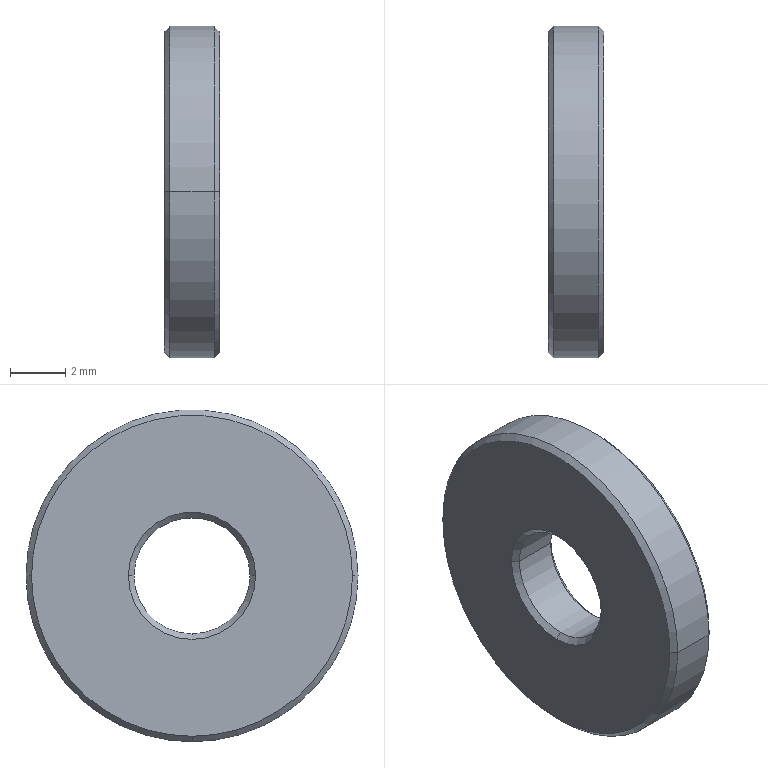Part | STEP file | BDQ-M4-D12-0.stp.STEP | 1 solid | 18 faces | box 2 x 12 x 12 mm | volume 196.45 mm3 | cone 12 | cylinder 4 | plane 2 | commonest cylinder face diameters 4.2 x2 12 x2
STEP:
#1=CARTESIAN_POINT('',(0.00000011,-2.3,0.));
#2=VERTEX_POINT('',#1);
#3=CARTESIAN_POINT('',(0.00000011,0.,-2.3));
#4=VERTEX_POINT('',#3);
#5=CARTESIAN_POINT('',(0.00000011,0.,0.));
#6=DIRECTION('',(1.,0.,0.));
#7=DIRECTION('',(0.,-1.,0.));
#8=AXIS2_PLACEMENT_3D('',#5,#6,#7);
#9=CIRCLE('',#8,2.3);
#10=EDGE_CURVE('',#2,#4,#9,.T.);
#11=ORIENTED_EDGE('',*,*,#10,.T.);
#12=CARTESIAN_POINT('',(0.00000011,2.3,0.));
#13=VERTEX_POINT('',#12);
#14=CARTESIAN_POINT('',(0.00000011,0.,0.));
#15=DIRECTION('',(1.,0.,0.));
#16=DIRECTION('',(0.,-1.,0.));
#17=AXIS2_PLACEMENT_3D('',#14,#15,#16);
#18=CIRCLE('',#17,2.3);
#19=EDGE_CURVE('',#4,#13,#18,.T.);
#20=ORIENTED_EDGE('',*,*,#19,.T.);
#21=CARTESIAN_POINT('',(0.00000011,0.,0.));
#22=DIRECTION('',(1.,0.,0.));
#23=DIRECTION('',(0.,1.,0.));
#24=AXIS2_PLACEMENT_3D('',#21,#22,#23);
#25=CIRCLE('',#24,2.3);
#26=EDGE_CURVE('',#13,#2,#25,.T.);
#27=ORIENTED_EDGE('',*,*,#26,.T.);
#28=EDGE_LOOP('',(#11,#20,#27));
#29=FACE_BOUND('',#28,.T.);
#30=CARTESIAN_POINT('',(0.000000236,5.8,0.));
#31=VERTEX_POINT('',#30);
#32=CARTESIAN_POINT('',(0.000000236,0.,-5.8));
#33=VERTEX_POINT('',#32);
#34=CARTESIAN_POINT('',(0.000000236,0.,0.));
#35=DIRECTION('',(-1.,0.,0.));
#36=DIRECTION('',(0.,1.,0.));
#37=AXIS2_PLACEMENT_3D('',#34,#35,#36);
#38=CIRCLE('',#37,5.8);
#39=EDGE_CURVE('',#31,#33,#38,.T.);
#40=ORIENTED_EDGE('',*,*,#39,.T.);
#41=CARTESIAN_POINT('',(0.000000236,-5.8,0.));
#42=VERTEX_POINT('',#41);
#43=CARTESIAN_POINT('',(0.000000236,0.,0.));
#44=DIRECTION('',(-1.,0.,0.));
#45=DIRECTION('',(0.,1.,0.));
#46=AXIS2_PLACEMENT_3D('',#43,#44,#45);
#47=CIRCLE('',#46,5.8);
#48=EDGE_CURVE('',#33,#42,#47,.T.);
#49=ORIENTED_EDGE('',*,*,#48,.T.);
#50=CARTESIAN_POINT('',(0.000000236,0.,0.));
#51=DIRECTION('',(-1.,0.,0.));
#52=DIRECTION('',(0.,-1.,0.));
#53=AXIS2_PLACEMENT_3D('',#50,#51,#52);
#54=CIRCLE('',#53,5.8);
#55=EDGE_CURVE('',#42,#31,#54,.T.);
#56=ORIENTED_EDGE('',*,*,#55,.T.);
#57=EDGE_LOOP('',(#40,#49,#56));
#58=FACE_OUTER_BOUND('',#57,.T.);
#59=CARTESIAN_POINT('',(0.,0.,0.));
#60=DIRECTION('',(1.,0.,0.));
#61=DIRECTION('',(0.,1.,0.));
#62=AXIS2_PLACEMENT_3D('',#59,#60,#61);
#63=PLANE('',#62);
#64=ADVANCED_FACE('',(#29,#58),#63,.F.);
#65=CARTESIAN_POINT('',(0.2,-6.,0.));
#66=VERTEX_POINT('',#65);
#67=CARTESIAN_POINT('',(0.000000318,-5.8,-0.000000001));
#68=DIRECTION('',(0.7071,-0.7071,0.000000001));
#69=VECTOR('',#68,1000.);
#70=LINE('',#67,#69);
#71=EDGE_CURVE('',#42,#66,#70,.T.);
#72=ORIENTED_EDGE('',*,*,#71,.T.);
#73=CARTESIAN_POINT('',(0.2,6.,0.));
#74=VERTEX_POINT('',#73);
#75=CARTESIAN_POINT('',(0.2,0.,0.));
#76=DIRECTION('',(-1.,0.,0.));
#77=DIRECTION('',(0.,-1.,0.));
#78=AXIS2_PLACEMENT_3D('',#75,#76,#77);
#79=CIRCLE('',#78,6.);
#80=EDGE_CURVE('',#66,#74,#79,.T.);
#81=ORIENTED_EDGE('',*,*,#80,.T.);
#82=CARTESIAN_POINT('',(0.000000318,5.8,0.000000001));
#83=DIRECTION('',(0.7071,0.7071,-0.000000001));
#84=VECTOR('',#83,1000.);
#85=LINE('',#82,#84);
#86=EDGE_CURVE('',#31,#74,#85,.T.);
#87=ORIENTED_EDGE('',*,*,#86,.F.);
#88=ORIENTED_EDGE('',*,*,#55,.F.);
#89=EDGE_LOOP('',(#72,#81,#87,#88));
#90=FACE_OUTER_BOUND('',#89,.T.);
#91=CARTESIAN_POINT('',(0.1,0.,0.));
#92=DIRECTION('',(1.,0.,0.));
#93=DIRECTION('',(0.,0.,-1.));
#94=AXIS2_PLACEMENT_3D('',#91,#92,#93);
#95=CONICAL_SURFACE('',#94,5.9,0.7854);
#96=ADVANCED_FACE('',(#90),#95,.T.);
#97=CARTESIAN_POINT('',(0.2,0.,-6.));
#98=VERTEX_POINT('',#97);
#99=CARTESIAN_POINT('',(0.1,0.,-5.9));
#100=DIRECTION('',(0.7071,0.,-0.7071));
#101=VECTOR('',#100,1000.);
#102=LINE('',#99,#101);
#103=EDGE_CURVE('',#33,#98,#102,.T.);
#104=ORIENTED_EDGE('',*,*,#103,.F.);
#105=ORIENTED_EDGE('',*,*,#39,.F.);
#106=ORIENTED_EDGE('',*,*,#86,.T.);
#107=CARTESIAN_POINT('',(0.2,0.,0.));
#108=DIRECTION('',(-1.,0.,0.));
#109=DIRECTION('',(0.,1.,0.));
#110=AXIS2_PLACEMENT_3D('',#107,#108,#109);
#111=CIRCLE('',#110,6.);
#112=EDGE_CURVE('',#74,#98,#111,.T.);
#113=ORIENTED_EDGE('',*,*,#112,.T.);
#114=EDGE_LOOP('',(#104,#105,#106,#113));
#115=FACE_OUTER_BOUND('',#114,.T.);
#116=CARTESIAN_POINT('',(0.1,0.,0.));
#117=DIRECTION('',(1.,0.,0.));
#118=DIRECTION('',(0.,0.,-1.));
#119=AXIS2_PLACEMENT_3D('',#116,#117,#118);
#120=CONICAL_SURFACE('',#119,5.9,0.7854);
#121=ADVANCED_FACE('',(#115),#120,.T.);
#122=CARTESIAN_POINT('',(1.8,-6.,0.));
#123=VERTEX_POINT('',#122);
#124=CARTESIAN_POINT('',(0.2,-6.,-0.000000001));
#125=DIRECTION('',(1.,0.,0.));
#126=VECTOR('',#125,1000.);
#127=LINE('',#124,#126);
#128=EDGE_CURVE('',#66,#123,#127,.T.);
#129=ORIENTED_EDGE('',*,*,#128,.F.);
#130=CARTESIAN_POINT('',(0.2,0.,0.));
#131=DIRECTION('',(-1.,0.,0.));
#132=DIRECTION('',(0.,1.,0.));
#133=AXIS2_PLACEMENT_3D('',#130,#131,#132);
#134=CIRCLE('',#133,6.);
#135=EDGE_CURVE('',#98,#66,#134,.T.);
#136=ORIENTED_EDGE('',*,*,#135,.F.);
#137=ORIENTED_EDGE('',*,*,#112,.F.);
#138=CARTESIAN_POINT('',(1.8,6.,0.));
#139=VERTEX_POINT('',#138);
#140=CARTESIAN_POINT('',(0.2,6.,0.000000001));
#141=DIRECTION('',(1.,0.,0.));
#142=VECTOR('',#141,1000.);
#143=LINE('',#140,#142);
#144=EDGE_CURVE('',#74,#139,#143,.T.);
#145=ORIENTED_EDGE('',*,*,#144,.T.);
#146=CARTESIAN_POINT('',(1.8,0.,-6.));
#147=VERTEX_POINT('',#146);
#148=CARTESIAN_POINT('',(1.8,0.,0.));
#149=DIRECTION('',(1.,0.,0.));
#150=DIRECTION('',(0.,-1.,0.));
#151=AXIS2_PLACEMENT_3D('',#148,#149,#150);
#152=CIRCLE('',#151,6.);
#153=EDGE_CURVE('',#147,#139,#152,.T.);
#154=ORIENTED_EDGE('',*,*,#153,.F.);
#155=CARTESIAN_POINT('',(1.8,0.,0.));
#156=DIRECTION('',(1.,0.,0.));
#157=DIRECTION('',(0.,-1.,0.));
#158=AXIS2_PLACEMENT_3D('',#155,#156,#157);
#159=CIRCLE('',#158,6.);
#160=EDGE_CURVE('',#123,#147,#159,.T.);
#161=ORIENTED_EDGE('',*,*,#160,.F.);
#162=EDGE_LOOP('',(#129,#136,#137,#145,#154,#161));
#163=FACE_OUTER_BOUND('',#162,.T.);
#164=CARTESIAN_POINT('',(0.,0.,0.));
#165=DIRECTION('',(1.,0.,0.));
#166=DIRECTION('',(0.,-1.,0.));
#167=AXIS2_PLACEMENT_3D('',#164,#165,#166);
#168=CYLINDRICAL_SURFACE('',#167,6.);
#169=ADVANCED_FACE('',(#163),#168,.T.);
#170=CARTESIAN_POINT('',(2.,0.,-5.8));
#171=VERTEX_POINT('',#170);
#172=CARTESIAN_POINT('',(1.9,0.,-5.9));
#173=DIRECTION('',(-0.7071,0.,-0.7071));
#174=VECTOR('',#173,1000.);
#175=LINE('',#172,#174);
#176=EDGE_CURVE('',#171,#147,#175,.T.);
#177=ORIENTED_EDGE('',*,*,#176,.F.);
#178=CARTESIAN_POINT('',(2.,-5.8,0.));
#179=VERTEX_POINT('',#178);
#180=CARTESIAN_POINT('',(2.,0.,0.));
#181=DIRECTION('',(1.,0.,0.));
#182=DIRECTION('',(0.,-1.,0.));
#183=AXIS2_PLACEMENT_3D('',#180,#181,#182);
#184=CIRCLE('',#183,5.8);
#185=EDGE_CURVE('',#179,#171,#184,.T.);
#186=ORIENTED_EDGE('',*,*,#185,.F.);
#187=CARTESIAN_POINT('',(2.,-5.8,-0.000000001));
#188=DIRECTION('',(-0.7071,-0.7071,0.000000001));
#189=VECTOR('',#188,1000.);
#190=LINE('',#187,#189);
#191=EDGE_CURVE('',#179,#123,#190,.T.);
#192=ORIENTED_EDGE('',*,*,#191,.T.);
#193=ORIENTED_EDGE('',*,*,#160,.T.);
#194=EDGE_LOOP('',(#177,#186,#192,#193));
#195=FACE_OUTER_BOUND('',#194,.T.);
#196=CARTESIAN_POINT('',(1.9,0.,0.));
#197=DIRECTION('',(-1.,0.,0.));
#198=DIRECTION('',(0.,0.,-1.));
#199=AXIS2_PLACEMENT_3D('',#196,#197,#198);
#200=CONICAL_SURFACE('',#199,5.9,0.7854);
#201=ADVANCED_FACE('',(#195),#200,.T.);
#202=CARTESIAN_POINT('',(2.,2.3,0.));
#203=VERTEX_POINT('',#202);
#204=CARTESIAN_POINT('',(2.,0.,-2.3));
#205=VERTEX_POINT('',#204);
#206=CARTESIAN_POINT('',(2.,0.,0.));
#207=DIRECTION('',(-1.,0.,0.));
#208=DIRECTION('',(0.,1.,0.));
#209=AXIS2_PLACEMENT_3D('',#206,#207,#208);
#210=CIRCLE('',#209,2.3);
#211=EDGE_CURVE('',#203,#205,#210,.T.);
#212=ORIENTED_EDGE('',*,*,#211,.T.);
#213=CARTESIAN_POINT('',(2.,-2.3,0.));
#214=VERTEX_POINT('',#213);
#215=CARTESIAN_POINT('',(2.,0.,0.));
#216=DIRECTION('',(-1.,0.,0.));
#217=DIRECTION('',(0.,1.,0.));
#218=AXIS2_PLACEMENT_3D('',#215,#216,#217);
#219=CIRCLE('',#218,2.3);
#220=EDGE_CURVE('',#205,#214,#219,.T.);
#221=ORIENTED_EDGE('',*,*,#220,.T.);
#222=CARTESIAN_POINT('',(2.,0.,0.));
#223=DIRECTION('',(-1.,0.,0.));
#224=DIRECTION('',(0.,-1.,0.));
#225=AXIS2_PLACEMENT_3D('',#222,#223,#224);
#226=CIRCLE('',#225,2.3);
#227=EDGE_CURVE('',#214,#203,#226,.T.);
#228=ORIENTED_EDGE('',*,*,#227,.T.);
#229=EDGE_LOOP('',(#212,#221,#228));
#230=FACE_BOUND('',#229,.T.);
#231=ORIENTED_EDGE('',*,*,#185,.T.);
#232=CARTESIAN_POINT('',(2.,5.8,0.));
#233=VERTEX_POINT('',#232);
#234=CARTESIAN_POINT('',(2.,0.,0.));
#235=DIRECTION('',(1.,0.,0.));
#236=DIRECTION('',(0.,-1.,0.));
#237=AXIS2_PLACEMENT_3D('',#234,#235,#236);
#238=CIRCLE('',#237,5.8);
#239=EDGE_CURVE('',#171,#233,#238,.T.);
#240=ORIENTED_EDGE('',*,*,#239,.T.);
#241=CARTESIAN_POINT('',(2.,0.,0.));
#242=DIRECTION('',(1.,0.,0.));
#243=DIRECTION('',(0.,1.,0.));
#244=AXIS2_PLACEMENT_3D('',#241,#242,#243);
#245=CIRCLE('',#244,5.8);
#246=EDGE_CURVE('',#233,#179,#245,.T.);
#247=ORIENTED_EDGE('',*,*,#246,.T.);
#248=EDGE_LOOP('',(#231,#240,#247));
#249=FACE_OUTER_BOUND('',#248,.T.);
#250=CARTESIAN_POINT('',(2.,0.,0.));
#251=DIRECTION('',(1.,0.,0.));
#252=DIRECTION('',(0.,1.,0.));
#253=AXIS2_PLACEMENT_3D('',#250,#251,#252);
#254=PLANE('',#253);
#255=ADVANCED_FACE('',(#230,#249),#254,.T.);
#256=CARTESIAN_POINT('',(2.,5.8,0.000000001));
#257=DIRECTION('',(-0.7071,0.7071,-0.000000001));
#258=VECTOR('',#257,1000.);
#259=LINE('',#256,#258);
#260=EDGE_CURVE('',#233,#139,#259,.T.);
#261=ORIENTED_EDGE('',*,*,#260,.T.);
#262=CARTESIAN_POINT('',(1.8,0.,0.));
#263=DIRECTION('',(1.,0.,0.));
#264=DIRECTION('',(0.,1.,0.));
#265=AXIS2_PLACEMENT_3D('',#262,#263,#264);
#266=CIRCLE('',#265,6.);
#267=EDGE_CURVE('',#139,#123,#266,.T.);
#268=ORIENTED_EDGE('',*,*,#267,.T.);
#269=ORIENTED_EDGE('',*,*,#191,.F.);
#270=ORIENTED_EDGE('',*,*,#246,.F.);
#271=EDGE_LOOP('',(#261,#268,#269,#270));
#272=FACE_OUTER_BOUND('',#271,.T.);
#273=CARTESIAN_POINT('',(1.9,0.,0.));
#274=DIRECTION('',(-1.,0.,0.));
#275=DIRECTION('',(0.,0.,-1.));
#276=AXIS2_PLACEMENT_3D('',#273,#274,#275);
#277=CONICAL_SURFACE('',#276,5.9,0.7854);
#278=ADVANCED_FACE('',(#272),#277,.T.);
#279=ORIENTED_EDGE('',*,*,#144,.F.);
#280=ORIENTED_EDGE('',*,*,#80,.F.);
#281=ORIENTED_EDGE('',*,*,#128,.T.);
#282=ORIENTED_EDGE('',*,*,#267,.F.);
#283=EDGE_LOOP('',(#279,#280,#281,#282));
#284=FACE_OUTER_BOUND('',#283,.T.);
#285=CARTESIAN_POINT('',(0.,0.,0.));
#286=DIRECTION('',(1.,0.,0.));
#287=DIRECTION('',(0.,-1.,0.));
#288=AXIS2_PLACEMENT_3D('',#285,#286,#287);
#289=CYLINDRICAL_SURFACE('',#288,6.);
#290=ADVANCED_FACE('',(#284),#289,.T.);
#291=CARTESIAN_POINT('',(1.8,-2.1,0.));
#292=VERTEX_POINT('',#291);
#293=CARTESIAN_POINT('',(2.,-2.3,-0.000000001));
#294=DIRECTION('',(-0.7071,0.7071,0.000000001));
#295=VECTOR('',#294,1000.);
#296=LINE('',#293,#295);
#297=EDGE_CURVE('',#214,#292,#296,.T.);
#298=ORIENTED_EDGE('',*,*,#297,.T.);
#299=CARTESIAN_POINT('',(1.8,2.1,0.));
#300=VERTEX_POINT('',#299);
#301=CARTESIAN_POINT('',(1.8,0.,0.));
#302=DIRECTION('',(-1.,0.,0.));
#303=DIRECTION('',(0.,-1.,0.));
#304=AXIS2_PLACEMENT_3D('',#301,#302,#303);
#305=CIRCLE('',#304,2.1);
#306=EDGE_CURVE('',#292,#300,#305,.T.);
#307=ORIENTED_EDGE('',*,*,#306,.T.);
#308=CARTESIAN_POINT('',(2.,2.3,0.000000001));
#309=DIRECTION('',(-0.7071,-0.7071,-0.000000001));
#310=VECTOR('',#309,1000.);
#311=LINE('',#308,#310);
#312=EDGE_CURVE('',#203,#300,#311,.T.);
#313=ORIENTED_EDGE('',*,*,#312,.F.);
#314=ORIENTED_EDGE('',*,*,#227,.F.);
#315=EDGE_LOOP('',(#298,#307,#313,#314));
#316=FACE_OUTER_BOUND('',#315,.T.);
#317=CARTESIAN_POINT('',(1.9,0.,0.));
#318=DIRECTION('',(1.,0.,0.));
#319=DIRECTION('',(0.,0.,-1.));
#320=AXIS2_PLACEMENT_3D('',#317,#318,#319);
#321=CONICAL_SURFACE('',#320,2.2,0.7854);
#322=ADVANCED_FACE('',(#316),#321,.F.);
#323=CARTESIAN_POINT('',(1.8,0.,-2.1));
#324=VERTEX_POINT('',#323);
#325=CARTESIAN_POINT('',(1.9,0.,-2.2));
#326=DIRECTION('',(0.7071,0.,-0.7071));
#327=VECTOR('',#326,1000.);
#328=LINE('',#325,#327);
#329=EDGE_CURVE('',#324,#205,#328,.T.);
#330=ORIENTED_EDGE('',*,*,#329,.F.);
#331=CARTESIAN_POINT('',(1.8,0.,0.));
#332=DIRECTION('',(-1.,0.,0.));
#333=DIRECTION('',(0.,1.,0.));
#334=AXIS2_PLACEMENT_3D('',#331,#332,#333);
#335=CIRCLE('',#334,2.1);
#336=EDGE_CURVE('',#324,#292,#335,.T.);
#337=ORIENTED_EDGE('',*,*,#336,.T.);
#338=ORIENTED_EDGE('',*,*,#297,.F.);
#339=ORIENTED_EDGE('',*,*,#220,.F.);
#340=EDGE_LOOP('',(#330,#337,#338,#339));
#341=FACE_OUTER_BOUND('',#340,.T.);
#342=CARTESIAN_POINT('',(1.9,0.,0.));
#343=DIRECTION('',(1.,0.,0.));
#344=DIRECTION('',(0.,0.,-1.));
#345=AXIS2_PLACEMENT_3D('',#342,#343,#344);
#346=CONICAL_SURFACE('',#345,2.2,0.7854);
#347=ADVANCED_FACE('',(#341),#346,.F.);
#348=CARTESIAN_POINT('',(0.2,2.1,0.));
#349=VERTEX_POINT('',#348);
#350=CARTESIAN_POINT('',(0.2,2.1,0.000000001));
#351=DIRECTION('',(1.,0.,0.));
#352=VECTOR('',#351,1000.);
#353=LINE('',#350,#352);
#354=EDGE_CURVE('',#349,#300,#353,.T.);
#355=ORIENTED_EDGE('',*,*,#354,.F.);
#356=CARTESIAN_POINT('',(0.2,0.,-2.1));
#357=VERTEX_POINT('',#356);
#358=CARTESIAN_POINT('',(0.2,0.,0.));
#359=DIRECTION('',(1.,0.,0.));
#360=DIRECTION('',(0.,-1.,0.));
#361=AXIS2_PLACEMENT_3D('',#358,#359,#360);
#362=CIRCLE('',#361,2.1);
#363=EDGE_CURVE('',#357,#349,#362,.T.);
#364=ORIENTED_EDGE('',*,*,#363,.F.);
#365=CARTESIAN_POINT('',(0.2,-2.1,0.));
#366=VERTEX_POINT('',#365);
#367=CARTESIAN_POINT('',(0.2,0.,0.));
#368=DIRECTION('',(1.,0.,0.));
#369=DIRECTION('',(0.,-1.,0.));
#370=AXIS2_PLACEMENT_3D('',#367,#368,#369);
#371=CIRCLE('',#370,2.1);
#372=EDGE_CURVE('',#366,#357,#371,.T.);
#373=ORIENTED_EDGE('',*,*,#372,.F.);
#374=CARTESIAN_POINT('',(0.2,-2.1,-0.000000001));
#375=DIRECTION('',(1.,0.,0.));
#376=VECTOR('',#375,1000.);
#377=LINE('',#374,#376);
#378=EDGE_CURVE('',#366,#292,#377,.T.);
#379=ORIENTED_EDGE('',*,*,#378,.T.);
#380=ORIENTED_EDGE('',*,*,#336,.F.);
#381=CARTESIAN_POINT('',(1.8,0.,0.));
#382=DIRECTION('',(-1.,0.,0.));
#383=DIRECTION('',(0.,1.,0.));
#384=AXIS2_PLACEMENT_3D('',#381,#382,#383);
#385=CIRCLE('',#384,2.1);
#386=EDGE_CURVE('',#300,#324,#385,.T.);
#387=ORIENTED_EDGE('',*,*,#386,.F.);
#388=EDGE_LOOP('',(#355,#364,#373,#379,#380,#387));
#389=FACE_OUTER_BOUND('',#388,.T.);
#390=CARTESIAN_POINT('',(0.,0.,0.));
#391=DIRECTION('',(1.,0.,0.));
#392=DIRECTION('',(0.,-1.,0.));
#393=AXIS2_PLACEMENT_3D('',#390,#391,#392);
#394=CYLINDRICAL_SURFACE('',#393,2.1);
#395=ADVANCED_FACE('',(#389),#394,.F.);
#396=ORIENTED_EDGE('',*,*,#378,.F.);
#397=CARTESIAN_POINT('',(0.2,0.,0.));
#398=DIRECTION('',(1.,0.,0.));
#399=DIRECTION('',(0.,1.,0.));
#400=AXIS2_PLACEMENT_3D('',#397,#398,#399);
#401=CIRCLE('',#400,2.1);
#402=EDGE_CURVE('',#349,#366,#401,.T.);
#403=ORIENTED_EDGE('',*,*,#402,.F.);
#404=ORIENTED_EDGE('',*,*,#354,.T.);
#405=ORIENTED_EDGE('',*,*,#306,.F.);
#406=EDGE_LOOP('',(#396,#403,#404,#405));
#407=FACE_OUTER_BOUND('',#406,.T.);
#408=CARTESIAN_POINT('',(0.,0.,0.));
#409=DIRECTION('',(1.,0.,0.));
#410=DIRECTION('',(0.,-1.,0.));
#411=AXIS2_PLACEMENT_3D('',#408,#409,#410);
#412=CYLINDRICAL_SURFACE('',#411,2.1);
#413=ADVANCED_FACE('',(#407),#412,.F.);
#414=CARTESIAN_POINT('',(-0.000000401,2.3,0.000000001));
#415=DIRECTION('',(0.7071,-0.7071,-0.000000001));
#416=VECTOR('',#415,1000.);
#417=LINE('',#414,#416);
#418=EDGE_CURVE('',#13,#349,#417,.T.);
#419=ORIENTED_EDGE('',*,*,#418,.T.);
#420=ORIENTED_EDGE('',*,*,#402,.T.);
#421=CARTESIAN_POINT('',(-0.000000401,-2.3,-0.000000001));
#422=DIRECTION('',(0.7071,0.7071,0.000000001));
#423=VECTOR('',#422,1000.);
#424=LINE('',#421,#423);
#425=EDGE_CURVE('',#2,#366,#424,.T.);
#426=ORIENTED_EDGE('',*,*,#425,.F.);
#427=ORIENTED_EDGE('',*,*,#26,.F.);
#428=EDGE_LOOP('',(#419,#420,#426,#427));
#429=FACE_OUTER_BOUND('',#428,.T.);
#430=CARTESIAN_POINT('',(0.1,0.,0.));
#431=DIRECTION('',(-1.,0.,0.));
#432=DIRECTION('',(0.,0.,-1.));
#433=AXIS2_PLACEMENT_3D('',#430,#431,#432);
#434=CONICAL_SURFACE('',#433,2.2,0.7854);
#435=ADVANCED_FACE('',(#429),#434,.F.);
#436=CARTESIAN_POINT('',(0.1,0.,-2.2));
#437=DIRECTION('',(-0.7071,0.,-0.7071));
#438=VECTOR('',#437,1000.);
#439=LINE('',#436,#438);
#440=EDGE_CURVE('',#357,#4,#439,.T.);
#441=ORIENTED_EDGE('',*,*,#440,.F.);
#442=ORIENTED_EDGE('',*,*,#363,.T.);
#443=ORIENTED_EDGE('',*,*,#418,.F.);
#444=ORIENTED_EDGE('',*,*,#19,.F.);
#445=EDGE_LOOP('',(#441,#442,#443,#444));
#446=FACE_OUTER_BOUND('',#445,.T.);
#447=CARTESIAN_POINT('',(0.1,0.,0.));
#448=DIRECTION('',(-1.,0.,0.));
#449=DIRECTION('',(0.,0.,-1.));
#450=AXIS2_PLACEMENT_3D('',#447,#448,#449);
#451=CONICAL_SURFACE('',#450,2.2,0.7854);
#452=ADVANCED_FACE('',(#446),#451,.F.);
#453=ORIENTED_EDGE('',*,*,#372,.T.);
#454=ORIENTED_EDGE('',*,*,#440,.T.);
#455=ORIENTED_EDGE('',*,*,#10,.F.);
#456=ORIENTED_EDGE('',*,*,#425,.T.);
#457=EDGE_LOOP('',(#453,#454,#455,#456));
#458=FACE_OUTER_BOUND('',#457,.T.);
#459=CARTESIAN_POINT('',(0.1,0.,0.));
#460=DIRECTION('',(-1.,0.,0.));
#461=DIRECTION('',(0.,0.,-1.));
#462=AXIS2_PLACEMENT_3D('',#459,#460,#461);
#463=CONICAL_SURFACE('',#462,2.2,0.7854);
#464=ADVANCED_FACE('',(#458),#463,.F.);
#465=ORIENTED_EDGE('',*,*,#386,.T.);
#466=ORIENTED_EDGE('',*,*,#329,.T.);
#467=ORIENTED_EDGE('',*,*,#211,.F.);
#468=ORIENTED_EDGE('',*,*,#312,.T.);
#469=EDGE_LOOP('',(#465,#466,#467,#468));
#470=FACE_OUTER_BOUND('',#469,.T.);
#471=CARTESIAN_POINT('',(1.9,0.,0.));
#472=DIRECTION('',(1.,0.,0.));
#473=DIRECTION('',(0.,0.,-1.));
#474=AXIS2_PLACEMENT_3D('',#471,#472,#473);
#475=CONICAL_SURFACE('',#474,2.2,0.7854);
#476=ADVANCED_FACE('',(#470),#475,.F.);
#477=ORIENTED_EDGE('',*,*,#239,.F.);
#478=ORIENTED_EDGE('',*,*,#176,.T.);
#479=ORIENTED_EDGE('',*,*,#153,.T.);
#480=ORIENTED_EDGE('',*,*,#260,.F.);
#481=EDGE_LOOP('',(#477,#478,#479,#480));
#482=FACE_OUTER_BOUND('',#481,.T.);
#483=CARTESIAN_POINT('',(1.9,0.,0.));
#484=DIRECTION('',(-1.,0.,0.));
#485=DIRECTION('',(0.,0.,-1.));
#486=AXIS2_PLACEMENT_3D('',#483,#484,#485);
#487=CONICAL_SURFACE('',#486,5.9,0.7854);
#488=ADVANCED_FACE('',(#482),#487,.T.);
#489=ORIENTED_EDGE('',*,*,#48,.F.);
#490=ORIENTED_EDGE('',*,*,#103,.T.);
#491=ORIENTED_EDGE('',*,*,#135,.T.);
#492=ORIENTED_EDGE('',*,*,#71,.F.);
#493=EDGE_LOOP('',(#489,#490,#491,#492));
#494=FACE_OUTER_BOUND('',#493,.T.);
#495=CARTESIAN_POINT('',(0.1,0.,0.));
#496=DIRECTION('',(1.,0.,0.));
#497=DIRECTION('',(0.,0.,-1.));
#498=AXIS2_PLACEMENT_3D('',#495,#496,#497);
#499=CONICAL_SURFACE('',#498,5.9,0.7854);
#500=ADVANCED_FACE('',(#494),#499,.T.);
#501=CLOSED_SHELL('',(#64,#96,#121,#169,#201,#255,#278,#290,#322,#347,#395,#413,#435,#452,#464,#476,#488,#500));
#502=MANIFOLD_SOLID_BREP('',#501);
#503=CARTESIAN_POINT('',(0.,0.,0.));
#504=DIRECTION('',(0.,0.,1.));
#505=DIRECTION('',(1.,0.,0.));
#506=AXIS2_PLACEMENT_3D('',#503,#504,#505);
#507=(LENGTH_UNIT()NAMED_UNIT(*)SI_UNIT(.MILLI.,.METRE.));
#508=UNCERTAINTY_MEASURE_WITH_UNIT(LENGTH_MEASURE(0.00001),#507,'','');
#509=(NAMED_UNIT(*)PLANE_ANGLE_UNIT()SI_UNIT($,.RADIAN.));
#510=(NAMED_UNIT(*)SI_UNIT($,.STERADIAN.)SOLID_ANGLE_UNIT());
#511=(GEOMETRIC_REPRESENTATION_CONTEXT(3)GLOBAL_UNCERTAINTY_ASSIGNED_CONTEXT((#508))GLOBAL_UNIT_ASSIGNED_CONTEXT((#507,#509,#510))REPRESENTATION_CONTEXT('',''));
#512=ADVANCED_BREP_SHAPE_REPRESENTATION('',(#502,#506),#511);